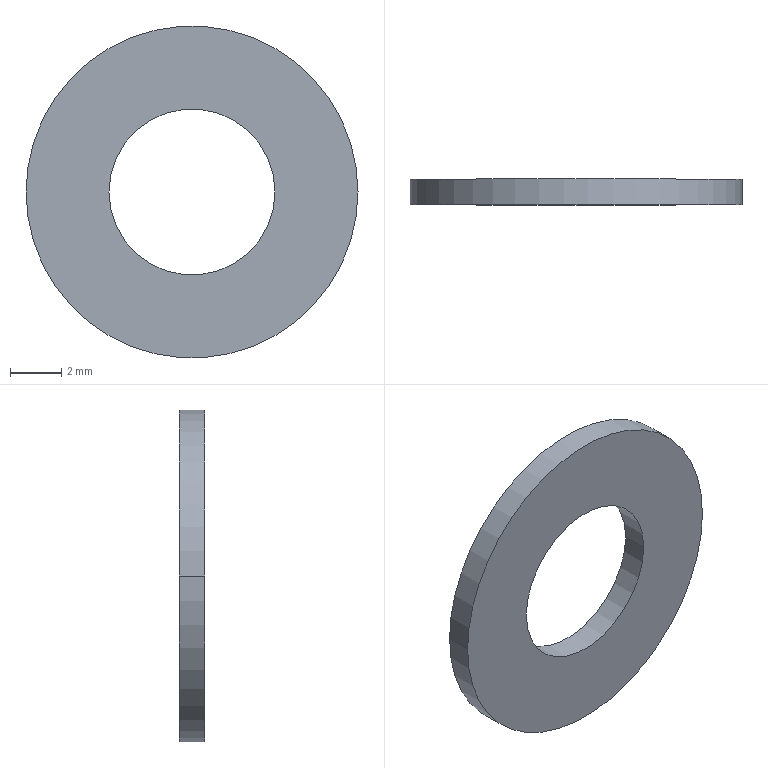Part | STEP file | ZZ21-M6-18 | 1 solid | 6 faces | box 13 x 1 x 13 mm | volume 99.549 mm3 | cylinder 4 | plane 2 | commonest cylinder face diameters 6.5 x2 13 x2
STEP:
#1=CARTESIAN_POINT('',(0.,0.,0.));
#2=DIRECTION('',(0.,0.,1.));
#3=DIRECTION('',(1.,0.,0.));
#4=AXIS2_PLACEMENT_3D('',#1,#2,#3);
#5=CARTESIAN_POINT('',(-3.25,0.,0.));
#6=VERTEX_POINT('',#5);
#7=CARTESIAN_POINT('',(-3.25,1.,0.));
#8=VERTEX_POINT('',#7);
#9=CARTESIAN_POINT('',(-3.25,0.,0.));
#10=DIRECTION('',(0.,1.,0.));
#11=VECTOR('',#10,1.);
#12=LINE('',#9,#11);
#13=CARTESIAN_POINT('',(0.,0.,0.));
#14=DIRECTION('',(0.,1.,0.));
#15=DIRECTION('',(-1.,0.,0.));
#16=AXIS2_PLACEMENT_3D('',#13,#14,#15);
#17=CYLINDRICAL_SURFACE('',#16,3.25);
#18=CARTESIAN_POINT('',(6.283,0.));
#19=DIRECTION('',(0.,1.));
#20=VECTOR('',#19,1.);
#21=LINE('',#18,#20);
#22=(GEOMETRIC_REPRESENTATION_CONTEXT(2)PARAMETRIC_REPRESENTATION_CONTEXT()REPRESENTATION_CONTEXT('',''));
#23=DEFINITIONAL_REPRESENTATION('',(#21),#22);
#24=PCURVE('',#17,#23);
#25=CARTESIAN_POINT('',(0.,0.,0.));
#26=DIRECTION('',(0.,1.,0.));
#27=DIRECTION('',(-1.,0.,0.));
#28=AXIS2_PLACEMENT_3D('',#25,#26,#27);
#29=CYLINDRICAL_SURFACE('',#28,3.25);
#30=CARTESIAN_POINT('',(0.,0.));
#31=DIRECTION('',(0.,1.));
#32=VECTOR('',#31,1.);
#33=LINE('',#30,#32);
#34=(GEOMETRIC_REPRESENTATION_CONTEXT(2)PARAMETRIC_REPRESENTATION_CONTEXT()REPRESENTATION_CONTEXT('',''));
#35=DEFINITIONAL_REPRESENTATION('',(#33),#34);
#36=PCURVE('',#29,#35);
#37=SURFACE_CURVE('',#12,(#24,#36),.PCURVE_S1.);
#38=EDGE_CURVE('',#6,#8,#37,.T.);
#39=ORIENTED_EDGE('',*,*,#38,.T.);
#40=CARTESIAN_POINT('',(3.25,1.,0.));
#41=VERTEX_POINT('',#40);
#42=CARTESIAN_POINT('',(0.,1.,0.));
#43=DIRECTION('',(0.,-1.,0.));
#44=DIRECTION('',(1.,0.,0.));
#45=AXIS2_PLACEMENT_3D('',#42,#43,#44);
#46=CIRCLE('',#45,3.25);
#47=CARTESIAN_POINT('',(9.425,1.));
#48=DIRECTION('',(-1.,0.));
#49=VECTOR('',#48,1.);
#50=LINE('',#47,#49);
#51=(GEOMETRIC_REPRESENTATION_CONTEXT(2)PARAMETRIC_REPRESENTATION_CONTEXT()REPRESENTATION_CONTEXT('',''));
#52=DEFINITIONAL_REPRESENTATION('',(#50),#51);
#53=PCURVE('',#17,#52);
#54=CARTESIAN_POINT('',(0.,1.,0.));
#55=DIRECTION('',(0.,1.,0.));
#56=DIRECTION('',(-1.,0.,0.));
#57=AXIS2_PLACEMENT_3D('',#54,#55,#56);
#58=PLANE('',#57);
#59=CARTESIAN_POINT('',(-3.25,0.));
#60=CARTESIAN_POINT('',(-3.25,5.629));
#61=CARTESIAN_POINT('',(1.625,2.815));
#62=CARTESIAN_POINT('',(6.5,0.));
#63=CARTESIAN_POINT('',(1.625,-2.815));
#64=CARTESIAN_POINT('',(-3.25,-5.629));
#65=CARTESIAN_POINT('',(-3.25,0.));
#66=(BOUNDED_CURVE()B_SPLINE_CURVE(2,(#59,#60,#61,#62,#63,#64,#65),.UNSPECIFIED.,.T.,.F.)B_SPLINE_CURVE_WITH_KNOTS((1,2,2,2,2,1),(-2.094,0.,2.094,4.189,6.283,8.378),.UNSPECIFIED.)CURVE()GEOMETRIC_REPRESENTATION_ITEM()RATIONAL_B_SPLINE_CURVE((1.,0.5,1.,0.5,1.,0.5,1.))REPRESENTATION_ITEM(''));
#67=(GEOMETRIC_REPRESENTATION_CONTEXT(2)PARAMETRIC_REPRESENTATION_CONTEXT()REPRESENTATION_CONTEXT('',''));
#68=DEFINITIONAL_REPRESENTATION('',(#66),#67);
#69=PCURVE('',#58,#68);
#70=SURFACE_CURVE('',#46,(#53,#69),.PCURVE_S1.);
#71=EDGE_CURVE('',#8,#41,#70,.T.);
#72=ORIENTED_EDGE('',*,*,#71,.T.);
#73=CARTESIAN_POINT('',(3.25,0.,0.));
#74=VERTEX_POINT('',#73);
#75=CARTESIAN_POINT('',(3.25,0.,0.));
#76=DIRECTION('',(0.,1.,0.));
#77=VECTOR('',#76,1.);
#78=LINE('',#75,#77);
#79=CARTESIAN_POINT('',(3.142,0.));
#80=DIRECTION('',(0.,1.));
#81=VECTOR('',#80,1.);
#82=LINE('',#79,#81);
#83=(GEOMETRIC_REPRESENTATION_CONTEXT(2)PARAMETRIC_REPRESENTATION_CONTEXT()REPRESENTATION_CONTEXT('',''));
#84=DEFINITIONAL_REPRESENTATION('',(#82),#83);
#85=PCURVE('',#17,#84);
#86=CARTESIAN_POINT('',(3.142,0.));
#87=DIRECTION('',(0.,1.));
#88=VECTOR('',#87,1.);
#89=LINE('',#86,#88);
#90=(GEOMETRIC_REPRESENTATION_CONTEXT(2)PARAMETRIC_REPRESENTATION_CONTEXT()REPRESENTATION_CONTEXT('',''));
#91=DEFINITIONAL_REPRESENTATION('',(#89),#90);
#92=PCURVE('',#29,#91);
#93=SURFACE_CURVE('',#78,(#85,#92),.PCURVE_S1.);
#94=EDGE_CURVE('',#74,#41,#93,.T.);
#95=ORIENTED_EDGE('',*,*,#94,.F.);
#96=CARTESIAN_POINT('',(0.,0.,0.));
#97=DIRECTION('',(0.,1.,0.));
#98=DIRECTION('',(-1.,0.,0.));
#99=AXIS2_PLACEMENT_3D('',#96,#97,#98);
#100=CIRCLE('',#99,3.25);
#101=CARTESIAN_POINT('',(0.,0.));
#102=DIRECTION('',(1.,0.));
#103=VECTOR('',#102,1.);
#104=LINE('',#101,#103);
#105=(GEOMETRIC_REPRESENTATION_CONTEXT(2)PARAMETRIC_REPRESENTATION_CONTEXT()REPRESENTATION_CONTEXT('',''));
#106=DEFINITIONAL_REPRESENTATION('',(#104),#105);
#107=PCURVE('',#17,#106);
#108=CARTESIAN_POINT('',(0.,0.,0.));
#109=DIRECTION('',(0.,-1.,0.));
#110=DIRECTION('',(1.,0.,0.));
#111=AXIS2_PLACEMENT_3D('',#108,#109,#110);
#112=PLANE('',#111);
#113=CARTESIAN_POINT('',(-3.25,0.));
#114=CARTESIAN_POINT('',(-3.25,5.629));
#115=CARTESIAN_POINT('',(1.625,2.815));
#116=CARTESIAN_POINT('',(6.5,0.));
#117=CARTESIAN_POINT('',(1.625,-2.815));
#118=CARTESIAN_POINT('',(-3.25,-5.629));
#119=CARTESIAN_POINT('',(-3.25,0.));
#120=(BOUNDED_CURVE()B_SPLINE_CURVE(2,(#113,#114,#115,#116,#117,#118,#119),.UNSPECIFIED.,.T.,.F.)B_SPLINE_CURVE_WITH_KNOTS((1,2,2,2,2,1),(-2.094,0.,2.094,4.189,6.283,8.378),.UNSPECIFIED.)CURVE()GEOMETRIC_REPRESENTATION_ITEM()RATIONAL_B_SPLINE_CURVE((1.,0.5,1.,0.5,1.,0.5,1.))REPRESENTATION_ITEM(''));
#121=(GEOMETRIC_REPRESENTATION_CONTEXT(2)PARAMETRIC_REPRESENTATION_CONTEXT()REPRESENTATION_CONTEXT('',''));
#122=DEFINITIONAL_REPRESENTATION('',(#120),#121);
#123=PCURVE('',#112,#122);
#124=SURFACE_CURVE('',#100,(#107,#123),.PCURVE_S1.);
#125=EDGE_CURVE('',#74,#6,#124,.T.);
#126=ORIENTED_EDGE('',*,*,#125,.T.);
#127=EDGE_LOOP('',(#39,#72,#95,#126));
#128=FACE_BOUND('',#127,.F.);
#129=ADVANCED_FACE('',(#128),#17,.F.);
#130=CARTESIAN_POINT('',(-6.5,0.,0.));
#131=VERTEX_POINT('',#130);
#132=CARTESIAN_POINT('',(6.5,0.,0.));
#133=VERTEX_POINT('',#132);
#134=CARTESIAN_POINT('',(0.,0.,0.));
#135=DIRECTION('',(0.,1.,0.));
#136=DIRECTION('',(-1.,0.,0.));
#137=AXIS2_PLACEMENT_3D('',#134,#135,#136);
#138=CIRCLE('',#137,6.5);
#139=CARTESIAN_POINT('',(0.,0.,0.));
#140=DIRECTION('',(0.,1.,0.));
#141=DIRECTION('',(-1.,0.,0.));
#142=AXIS2_PLACEMENT_3D('',#139,#140,#141);
#143=CYLINDRICAL_SURFACE('',#142,6.5);
#144=CARTESIAN_POINT('',(0.,0.));
#145=DIRECTION('',(1.,0.));
#146=VECTOR('',#145,1.);
#147=LINE('',#144,#146);
#148=(GEOMETRIC_REPRESENTATION_CONTEXT(2)PARAMETRIC_REPRESENTATION_CONTEXT()REPRESENTATION_CONTEXT('',''));
#149=DEFINITIONAL_REPRESENTATION('',(#147),#148);
#150=PCURVE('',#143,#149);
#151=CARTESIAN_POINT('',(-6.5,0.));
#152=CARTESIAN_POINT('',(-6.5,11.258));
#153=CARTESIAN_POINT('',(3.25,5.629));
#154=CARTESIAN_POINT('',(13.,0.));
#155=CARTESIAN_POINT('',(3.25,-5.629));
#156=CARTESIAN_POINT('',(-6.5,-11.258));
#157=CARTESIAN_POINT('',(-6.5,0.));
#158=(BOUNDED_CURVE()B_SPLINE_CURVE(2,(#151,#152,#153,#154,#155,#156,#157),.UNSPECIFIED.,.T.,.F.)B_SPLINE_CURVE_WITH_KNOTS((1,2,2,2,2,1),(-2.094,0.,2.094,4.189,6.283,8.378),.UNSPECIFIED.)CURVE()GEOMETRIC_REPRESENTATION_ITEM()RATIONAL_B_SPLINE_CURVE((1.,0.5,1.,0.5,1.,0.5,1.))REPRESENTATION_ITEM(''));
#159=(GEOMETRIC_REPRESENTATION_CONTEXT(2)PARAMETRIC_REPRESENTATION_CONTEXT()REPRESENTATION_CONTEXT('',''));
#160=DEFINITIONAL_REPRESENTATION('',(#158),#159);
#161=PCURVE('',#112,#160);
#162=SURFACE_CURVE('',#138,(#150,#161),.PCURVE_S1.);
#163=EDGE_CURVE('',#131,#133,#162,.T.);
#164=ORIENTED_EDGE('',*,*,#163,.T.);
#165=CARTESIAN_POINT('',(6.5,1.,0.));
#166=VERTEX_POINT('',#165);
#167=CARTESIAN_POINT('',(6.5,0.,0.));
#168=DIRECTION('',(0.,1.,0.));
#169=VECTOR('',#168,1.);
#170=LINE('',#167,#169);
#171=CARTESIAN_POINT('',(3.142,0.));
#172=DIRECTION('',(0.,1.));
#173=VECTOR('',#172,1.);
#174=LINE('',#171,#173);
#175=(GEOMETRIC_REPRESENTATION_CONTEXT(2)PARAMETRIC_REPRESENTATION_CONTEXT()REPRESENTATION_CONTEXT('',''));
#176=DEFINITIONAL_REPRESENTATION('',(#174),#175);
#177=PCURVE('',#143,#176);
#178=CARTESIAN_POINT('',(0.,0.,0.));
#179=DIRECTION('',(0.,1.,0.));
#180=DIRECTION('',(-1.,0.,0.));
#181=AXIS2_PLACEMENT_3D('',#178,#179,#180);
#182=CYLINDRICAL_SURFACE('',#181,6.5);
#183=CARTESIAN_POINT('',(3.142,0.));
#184=DIRECTION('',(0.,1.));
#185=VECTOR('',#184,1.);
#186=LINE('',#183,#185);
#187=(GEOMETRIC_REPRESENTATION_CONTEXT(2)PARAMETRIC_REPRESENTATION_CONTEXT()REPRESENTATION_CONTEXT('',''));
#188=DEFINITIONAL_REPRESENTATION('',(#186),#187);
#189=PCURVE('',#182,#188);
#190=SURFACE_CURVE('',#170,(#177,#189),.PCURVE_S1.);
#191=EDGE_CURVE('',#133,#166,#190,.T.);
#192=ORIENTED_EDGE('',*,*,#191,.T.);
#193=CARTESIAN_POINT('',(-6.5,1.,0.));
#194=VERTEX_POINT('',#193);
#195=CARTESIAN_POINT('',(0.,1.,0.));
#196=DIRECTION('',(0.,-1.,0.));
#197=DIRECTION('',(1.,0.,0.));
#198=AXIS2_PLACEMENT_3D('',#195,#196,#197);
#199=CIRCLE('',#198,6.5);
#200=CARTESIAN_POINT('',(3.142,1.));
#201=DIRECTION('',(-1.,0.));
#202=VECTOR('',#201,1.);
#203=LINE('',#200,#202);
#204=(GEOMETRIC_REPRESENTATION_CONTEXT(2)PARAMETRIC_REPRESENTATION_CONTEXT()REPRESENTATION_CONTEXT('',''));
#205=DEFINITIONAL_REPRESENTATION('',(#203),#204);
#206=PCURVE('',#143,#205);
#207=CARTESIAN_POINT('',(-6.5,0.));
#208=CARTESIAN_POINT('',(-6.5,11.258));
#209=CARTESIAN_POINT('',(3.25,5.629));
#210=CARTESIAN_POINT('',(13.,0.));
#211=CARTESIAN_POINT('',(3.25,-5.629));
#212=CARTESIAN_POINT('',(-6.5,-11.258));
#213=CARTESIAN_POINT('',(-6.5,0.));
#214=(BOUNDED_CURVE()B_SPLINE_CURVE(2,(#207,#208,#209,#210,#211,#212,#213),.UNSPECIFIED.,.T.,.F.)B_SPLINE_CURVE_WITH_KNOTS((1,2,2,2,2,1),(-2.094,0.,2.094,4.189,6.283,8.378),.UNSPECIFIED.)CURVE()GEOMETRIC_REPRESENTATION_ITEM()RATIONAL_B_SPLINE_CURVE((1.,0.5,1.,0.5,1.,0.5,1.))REPRESENTATION_ITEM(''));
#215=(GEOMETRIC_REPRESENTATION_CONTEXT(2)PARAMETRIC_REPRESENTATION_CONTEXT()REPRESENTATION_CONTEXT('',''));
#216=DEFINITIONAL_REPRESENTATION('',(#214),#215);
#217=PCURVE('',#58,#216);
#218=SURFACE_CURVE('',#199,(#206,#217),.PCURVE_S1.);
#219=EDGE_CURVE('',#166,#194,#218,.T.);
#220=ORIENTED_EDGE('',*,*,#219,.T.);
#221=CARTESIAN_POINT('',(-6.5,0.,0.));
#222=DIRECTION('',(0.,1.,0.));
#223=VECTOR('',#222,1.);
#224=LINE('',#221,#223);
#225=CARTESIAN_POINT('',(0.,0.));
#226=DIRECTION('',(0.,1.));
#227=VECTOR('',#226,1.);
#228=LINE('',#225,#227);
#229=(GEOMETRIC_REPRESENTATION_CONTEXT(2)PARAMETRIC_REPRESENTATION_CONTEXT()REPRESENTATION_CONTEXT('',''));
#230=DEFINITIONAL_REPRESENTATION('',(#228),#229);
#231=PCURVE('',#143,#230);
#232=CARTESIAN_POINT('',(6.283,0.));
#233=DIRECTION('',(0.,1.));
#234=VECTOR('',#233,1.);
#235=LINE('',#232,#234);
#236=(GEOMETRIC_REPRESENTATION_CONTEXT(2)PARAMETRIC_REPRESENTATION_CONTEXT()REPRESENTATION_CONTEXT('',''));
#237=DEFINITIONAL_REPRESENTATION('',(#235),#236);
#238=PCURVE('',#182,#237);
#239=SURFACE_CURVE('',#224,(#231,#238),.PCURVE_S1.);
#240=EDGE_CURVE('',#131,#194,#239,.T.);
#241=ORIENTED_EDGE('',*,*,#240,.F.);
#242=EDGE_LOOP('',(#164,#192,#220,#241));
#243=FACE_BOUND('',#242,.T.);
#244=ADVANCED_FACE('',(#243),#143,.T.);
#245=ORIENTED_EDGE('',*,*,#71,.T.);
#246=CARTESIAN_POINT('',(0.,1.,0.));
#247=DIRECTION('',(0.,-1.,0.));
#248=DIRECTION('',(1.,0.,0.));
#249=AXIS2_PLACEMENT_3D('',#246,#247,#248);
#250=CIRCLE('',#249,3.25);
#251=CARTESIAN_POINT('',(-3.25,0.));
#252=CARTESIAN_POINT('',(-3.25,5.629));
#253=CARTESIAN_POINT('',(1.625,2.815));
#254=CARTESIAN_POINT('',(6.5,0.));
#255=CARTESIAN_POINT('',(1.625,-2.815));
#256=CARTESIAN_POINT('',(-3.25,-5.629));
#257=CARTESIAN_POINT('',(-3.25,0.));
#258=(BOUNDED_CURVE()B_SPLINE_CURVE(2,(#251,#252,#253,#254,#255,#256,#257),.UNSPECIFIED.,.T.,.F.)B_SPLINE_CURVE_WITH_KNOTS((1,2,2,2,2,1),(-2.094,0.,2.094,4.189,6.283,8.378),.UNSPECIFIED.)CURVE()GEOMETRIC_REPRESENTATION_ITEM()RATIONAL_B_SPLINE_CURVE((1.,0.5,1.,0.5,1.,0.5,1.))REPRESENTATION_ITEM(''));
#259=(GEOMETRIC_REPRESENTATION_CONTEXT(2)PARAMETRIC_REPRESENTATION_CONTEXT()REPRESENTATION_CONTEXT('',''));
#260=DEFINITIONAL_REPRESENTATION('',(#258),#259);
#261=PCURVE('',#58,#260);
#262=CARTESIAN_POINT('',(3.142,1.));
#263=DIRECTION('',(-1.,0.));
#264=VECTOR('',#263,1.);
#265=LINE('',#262,#264);
#266=(GEOMETRIC_REPRESENTATION_CONTEXT(2)PARAMETRIC_REPRESENTATION_CONTEXT()REPRESENTATION_CONTEXT('',''));
#267=DEFINITIONAL_REPRESENTATION('',(#265),#266);
#268=PCURVE('',#29,#267);
#269=SURFACE_CURVE('',#250,(#261,#268),.PCURVE_S1.);
#270=EDGE_CURVE('',#41,#8,#269,.T.);
#271=ORIENTED_EDGE('',*,*,#270,.T.);
#272=EDGE_LOOP('',(#245,#271));
#273=FACE_BOUND('',#272,.T.);
#274=CARTESIAN_POINT('',(0.,1.,0.));
#275=DIRECTION('',(0.,-1.,0.));
#276=DIRECTION('',(1.,0.,0.));
#277=AXIS2_PLACEMENT_3D('',#274,#275,#276);
#278=CIRCLE('',#277,6.5);
#279=CARTESIAN_POINT('',(-6.5,0.));
#280=CARTESIAN_POINT('',(-6.5,11.258));
#281=CARTESIAN_POINT('',(3.25,5.629));
#282=CARTESIAN_POINT('',(13.,0.));
#283=CARTESIAN_POINT('',(3.25,-5.629));
#284=CARTESIAN_POINT('',(-6.5,-11.258));
#285=CARTESIAN_POINT('',(-6.5,0.));
#286=(BOUNDED_CURVE()B_SPLINE_CURVE(2,(#279,#280,#281,#282,#283,#284,#285),.UNSPECIFIED.,.T.,.F.)B_SPLINE_CURVE_WITH_KNOTS((1,2,2,2,2,1),(-2.094,0.,2.094,4.189,6.283,8.378),.UNSPECIFIED.)CURVE()GEOMETRIC_REPRESENTATION_ITEM()RATIONAL_B_SPLINE_CURVE((1.,0.5,1.,0.5,1.,0.5,1.))REPRESENTATION_ITEM(''));
#287=(GEOMETRIC_REPRESENTATION_CONTEXT(2)PARAMETRIC_REPRESENTATION_CONTEXT()REPRESENTATION_CONTEXT('',''));
#288=DEFINITIONAL_REPRESENTATION('',(#286),#287);
#289=PCURVE('',#58,#288);
#290=CARTESIAN_POINT('',(9.425,1.));
#291=DIRECTION('',(-1.,0.));
#292=VECTOR('',#291,1.);
#293=LINE('',#290,#292);
#294=(GEOMETRIC_REPRESENTATION_CONTEXT(2)PARAMETRIC_REPRESENTATION_CONTEXT()REPRESENTATION_CONTEXT('',''));
#295=DEFINITIONAL_REPRESENTATION('',(#293),#294);
#296=PCURVE('',#182,#295);
#297=SURFACE_CURVE('',#278,(#289,#296),.PCURVE_S1.);
#298=EDGE_CURVE('',#194,#166,#297,.T.);
#299=ORIENTED_EDGE('',*,*,#298,.F.);
#300=ORIENTED_EDGE('',*,*,#219,.F.);
#301=EDGE_LOOP('',(#299,#300));
#302=FACE_BOUND('',#301,.T.);
#303=ADVANCED_FACE('',(#273,#302),#58,.T.);
#304=CARTESIAN_POINT('',(0.,0.,0.));
#305=DIRECTION('',(0.,1.,0.));
#306=DIRECTION('',(-1.,0.,0.));
#307=AXIS2_PLACEMENT_3D('',#304,#305,#306);
#308=CIRCLE('',#307,3.25);
#309=CARTESIAN_POINT('',(-3.25,0.));
#310=CARTESIAN_POINT('',(-3.25,5.629));
#311=CARTESIAN_POINT('',(1.625,2.815));
#312=CARTESIAN_POINT('',(6.5,0.));
#313=CARTESIAN_POINT('',(1.625,-2.815));
#314=CARTESIAN_POINT('',(-3.25,-5.629));
#315=CARTESIAN_POINT('',(-3.25,0.));
#316=(BOUNDED_CURVE()B_SPLINE_CURVE(2,(#309,#310,#311,#312,#313,#314,#315),.UNSPECIFIED.,.T.,.F.)B_SPLINE_CURVE_WITH_KNOTS((1,2,2,2,2,1),(-2.094,0.,2.094,4.189,6.283,8.378),.UNSPECIFIED.)CURVE()GEOMETRIC_REPRESENTATION_ITEM()RATIONAL_B_SPLINE_CURVE((1.,0.5,1.,0.5,1.,0.5,1.))REPRESENTATION_ITEM(''));
#317=(GEOMETRIC_REPRESENTATION_CONTEXT(2)PARAMETRIC_REPRESENTATION_CONTEXT()REPRESENTATION_CONTEXT('',''));
#318=DEFINITIONAL_REPRESENTATION('',(#316),#317);
#319=PCURVE('',#112,#318);
#320=CARTESIAN_POINT('',(0.,0.));
#321=DIRECTION('',(1.,0.));
#322=VECTOR('',#321,1.);
#323=LINE('',#320,#322);
#324=(GEOMETRIC_REPRESENTATION_CONTEXT(2)PARAMETRIC_REPRESENTATION_CONTEXT()REPRESENTATION_CONTEXT('',''));
#325=DEFINITIONAL_REPRESENTATION('',(#323),#324);
#326=PCURVE('',#29,#325);
#327=SURFACE_CURVE('',#308,(#319,#326),.PCURVE_S1.);
#328=EDGE_CURVE('',#6,#74,#327,.T.);
#329=ORIENTED_EDGE('',*,*,#328,.T.);
#330=ORIENTED_EDGE('',*,*,#125,.T.);
#331=EDGE_LOOP('',(#329,#330));
#332=FACE_BOUND('',#331,.T.);
#333=ORIENTED_EDGE('',*,*,#163,.F.);
#334=CARTESIAN_POINT('',(0.,0.,0.));
#335=DIRECTION('',(0.,1.,0.));
#336=DIRECTION('',(-1.,0.,0.));
#337=AXIS2_PLACEMENT_3D('',#334,#335,#336);
#338=CIRCLE('',#337,6.5);
#339=CARTESIAN_POINT('',(-6.5,0.));
#340=CARTESIAN_POINT('',(-6.5,11.258));
#341=CARTESIAN_POINT('',(3.25,5.629));
#342=CARTESIAN_POINT('',(13.,0.));
#343=CARTESIAN_POINT('',(3.25,-5.629));
#344=CARTESIAN_POINT('',(-6.5,-11.258));
#345=CARTESIAN_POINT('',(-6.5,0.));
#346=(BOUNDED_CURVE()B_SPLINE_CURVE(2,(#339,#340,#341,#342,#343,#344,#345),.UNSPECIFIED.,.T.,.F.)B_SPLINE_CURVE_WITH_KNOTS((1,2,2,2,2,1),(-2.094,0.,2.094,4.189,6.283,8.378),.UNSPECIFIED.)CURVE()GEOMETRIC_REPRESENTATION_ITEM()RATIONAL_B_SPLINE_CURVE((1.,0.5,1.,0.5,1.,0.5,1.))REPRESENTATION_ITEM(''));
#347=(GEOMETRIC_REPRESENTATION_CONTEXT(2)PARAMETRIC_REPRESENTATION_CONTEXT()REPRESENTATION_CONTEXT('',''));
#348=DEFINITIONAL_REPRESENTATION('',(#346),#347);
#349=PCURVE('',#112,#348);
#350=CARTESIAN_POINT('',(0.,0.));
#351=DIRECTION('',(1.,0.));
#352=VECTOR('',#351,1.);
#353=LINE('',#350,#352);
#354=(GEOMETRIC_REPRESENTATION_CONTEXT(2)PARAMETRIC_REPRESENTATION_CONTEXT()REPRESENTATION_CONTEXT('',''));
#355=DEFINITIONAL_REPRESENTATION('',(#353),#354);
#356=PCURVE('',#182,#355);
#357=SURFACE_CURVE('',#338,(#349,#356),.PCURVE_S1.);
#358=EDGE_CURVE('',#133,#131,#357,.T.);
#359=ORIENTED_EDGE('',*,*,#358,.F.);
#360=EDGE_LOOP('',(#333,#359));
#361=FACE_BOUND('',#360,.T.);
#362=ADVANCED_FACE('',(#332,#361),#112,.T.);
#363=ORIENTED_EDGE('',*,*,#191,.F.);
#364=ORIENTED_EDGE('',*,*,#358,.T.);
#365=ORIENTED_EDGE('',*,*,#240,.T.);
#366=ORIENTED_EDGE('',*,*,#298,.T.);
#367=EDGE_LOOP('',(#363,#364,#365,#366));
#368=FACE_BOUND('',#367,.T.);
#369=ADVANCED_FACE('',(#368),#182,.T.);
#370=ORIENTED_EDGE('',*,*,#270,.T.);
#371=ORIENTED_EDGE('',*,*,#38,.F.);
#372=ORIENTED_EDGE('',*,*,#328,.T.);
#373=ORIENTED_EDGE('',*,*,#94,.T.);
#374=EDGE_LOOP('',(#370,#371,#372,#373));
#375=FACE_BOUND('',#374,.F.);
#376=ADVANCED_FACE('',(#375),#29,.F.);
#377=CLOSED_SHELL('',(#129,#244,#303,#362,#369,#376));
#378=MANIFOLD_SOLID_BREP('',#377);
#379=(LENGTH_UNIT()NAMED_UNIT(*)SI_UNIT(.MILLI.,.METRE.));
#380=UNCERTAINTY_MEASURE_WITH_UNIT(LENGTH_MEASURE(0.0000001),#379,'','');
#381=(NAMED_UNIT(*)PLANE_ANGLE_UNIT()SI_UNIT($,.RADIAN.));
#382=(NAMED_UNIT(*)SI_UNIT($,.STERADIAN.)SOLID_ANGLE_UNIT());
#383=(GEOMETRIC_REPRESENTATION_CONTEXT(3)GLOBAL_UNCERTAINTY_ASSIGNED_CONTEXT((#380))GLOBAL_UNIT_ASSIGNED_CONTEXT((#379,#381,#382))REPRESENTATION_CONTEXT('',''));
#384=ADVANCED_BREP_SHAPE_REPRESENTATION('',(#4,#378),#383);